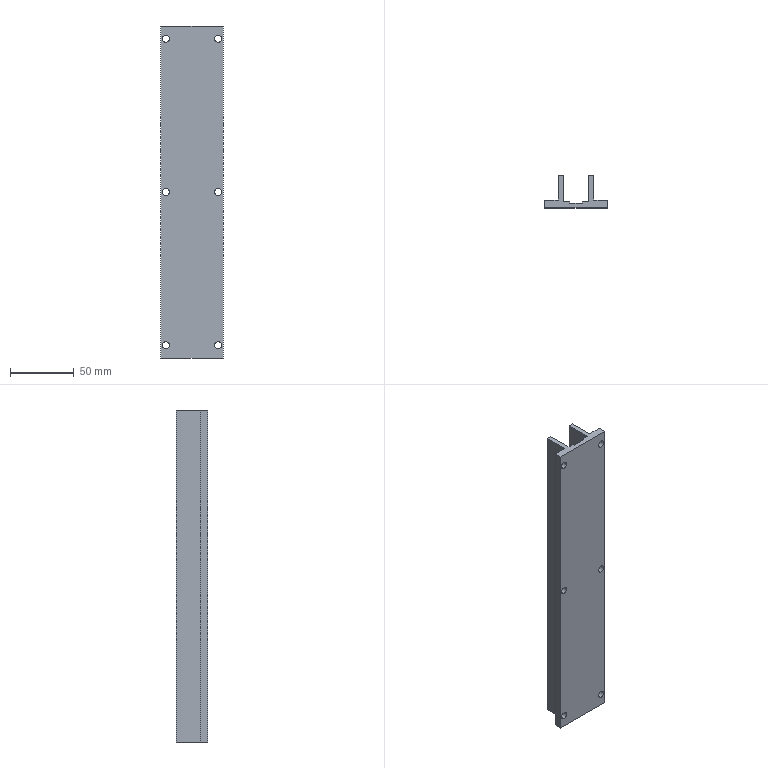Part | SolidWorks | features BaseBody 1 | 1 solid | 30 faces | box 49 x 25 x 260 mm | volume 106005 mm3 | plane 18 | cylinder 12 | commonest cylinder face diameters 5.5 x12
STEP:
#1=CARTESIAN_POINT('',(20.5,0.,252.75));
#2=VERTEX_POINT('',#1);
#3=CARTESIAN_POINT('',(20.5,0.,247.25));
#4=VERTEX_POINT('',#3);
#5=CARTESIAN_POINT('',(20.5,0.,250.));
#6=DIRECTION('',(0.,-1.,0.));
#7=DIRECTION('',(0.,0.,1.));
#8=AXIS2_PLACEMENT_3D('',#5,#6,#7);
#9=CIRCLE('',#8,2.75);
#10=EDGE_CURVE('',#2,#4,#9,.T.);
#11=ORIENTED_EDGE('',*,*,#10,.T.);
#12=CARTESIAN_POINT('',(20.5,6.,247.25));
#13=VERTEX_POINT('',#12);
#14=CARTESIAN_POINT('',(20.5,6.,247.25));
#15=DIRECTION('',(0.,1.,0.));
#16=VECTOR('',#15,1000.);
#17=LINE('',#14,#16);
#18=EDGE_CURVE('',#4,#13,#17,.T.);
#19=ORIENTED_EDGE('',*,*,#18,.T.);
#20=CARTESIAN_POINT('',(20.5,6.,252.75));
#21=VERTEX_POINT('',#20);
#22=CARTESIAN_POINT('',(20.5,6.,250.));
#23=DIRECTION('',(0.,-1.,0.));
#24=DIRECTION('',(0.,0.,1.));
#25=AXIS2_PLACEMENT_3D('',#22,#23,#24);
#26=CIRCLE('',#25,2.75);
#27=EDGE_CURVE('',#21,#13,#26,.T.);
#28=ORIENTED_EDGE('',*,*,#27,.F.);
#29=CARTESIAN_POINT('',(20.5,6.,252.75));
#30=DIRECTION('',(0.,1.,0.));
#31=VECTOR('',#30,1000.);
#32=LINE('',#29,#31);
#33=EDGE_CURVE('',#2,#21,#32,.T.);
#34=ORIENTED_EDGE('',*,*,#33,.F.);
#35=EDGE_LOOP('',(#11,#19,#28,#34));
#36=FACE_OUTER_BOUND('',#35,.T.);
#37=CARTESIAN_POINT('',(20.5,6.,250.));
#38=DIRECTION('',(0.,1.,0.));
#39=DIRECTION('',(0.,0.,1.));
#40=AXIS2_PLACEMENT_3D('',#37,#38,#39);
#41=CYLINDRICAL_SURFACE('',#40,2.75);
#42=ADVANCED_FACE('',(#36),#41,.F.);
#43=CARTESIAN_POINT('',(20.5,0.,132.75));
#44=VERTEX_POINT('',#43);
#45=CARTESIAN_POINT('',(20.5,0.,127.25));
#46=VERTEX_POINT('',#45);
#47=CARTESIAN_POINT('',(20.5,0.,130.));
#48=DIRECTION('',(0.,-1.,0.));
#49=DIRECTION('',(0.,0.,1.));
#50=AXIS2_PLACEMENT_3D('',#47,#48,#49);
#51=CIRCLE('',#50,2.75);
#52=EDGE_CURVE('',#44,#46,#51,.T.);
#53=ORIENTED_EDGE('',*,*,#52,.T.);
#54=CARTESIAN_POINT('',(20.5,6.,127.25));
#55=VERTEX_POINT('',#54);
#56=CARTESIAN_POINT('',(20.5,6.,127.25));
#57=DIRECTION('',(0.,1.,0.));
#58=VECTOR('',#57,1000.);
#59=LINE('',#56,#58);
#60=EDGE_CURVE('',#46,#55,#59,.T.);
#61=ORIENTED_EDGE('',*,*,#60,.T.);
#62=CARTESIAN_POINT('',(20.5,6.,132.75));
#63=VERTEX_POINT('',#62);
#64=CARTESIAN_POINT('',(20.5,6.,130.));
#65=DIRECTION('',(0.,-1.,0.));
#66=DIRECTION('',(0.,0.,1.));
#67=AXIS2_PLACEMENT_3D('',#64,#65,#66);
#68=CIRCLE('',#67,2.75);
#69=EDGE_CURVE('',#63,#55,#68,.T.);
#70=ORIENTED_EDGE('',*,*,#69,.F.);
#71=CARTESIAN_POINT('',(20.5,6.,132.75));
#72=DIRECTION('',(0.,1.,0.));
#73=VECTOR('',#72,1000.);
#74=LINE('',#71,#73);
#75=EDGE_CURVE('',#44,#63,#74,.T.);
#76=ORIENTED_EDGE('',*,*,#75,.F.);
#77=EDGE_LOOP('',(#53,#61,#70,#76));
#78=FACE_OUTER_BOUND('',#77,.T.);
#79=CARTESIAN_POINT('',(20.5,6.,130.));
#80=DIRECTION('',(0.,1.,0.));
#81=DIRECTION('',(0.,0.,1.));
#82=AXIS2_PLACEMENT_3D('',#79,#80,#81);
#83=CYLINDRICAL_SURFACE('',#82,2.75);
#84=ADVANCED_FACE('',(#78),#83,.F.);
#85=CARTESIAN_POINT('',(20.5,0.,12.75));
#86=VERTEX_POINT('',#85);
#87=CARTESIAN_POINT('',(20.5,0.,7.25));
#88=VERTEX_POINT('',#87);
#89=CARTESIAN_POINT('',(20.5,0.,10.));
#90=DIRECTION('',(0.,-1.,0.));
#91=DIRECTION('',(0.,0.,1.));
#92=AXIS2_PLACEMENT_3D('',#89,#90,#91);
#93=CIRCLE('',#92,2.75);
#94=EDGE_CURVE('',#86,#88,#93,.T.);
#95=ORIENTED_EDGE('',*,*,#94,.T.);
#96=CARTESIAN_POINT('',(20.5,6.,7.25));
#97=VERTEX_POINT('',#96);
#98=CARTESIAN_POINT('',(20.5,6.,7.25));
#99=DIRECTION('',(0.,1.,0.));
#100=VECTOR('',#99,1000.);
#101=LINE('',#98,#100);
#102=EDGE_CURVE('',#88,#97,#101,.T.);
#103=ORIENTED_EDGE('',*,*,#102,.T.);
#104=CARTESIAN_POINT('',(20.5,6.,12.75));
#105=VERTEX_POINT('',#104);
#106=CARTESIAN_POINT('',(20.5,6.,10.));
#107=DIRECTION('',(0.,-1.,0.));
#108=DIRECTION('',(0.,0.,1.));
#109=AXIS2_PLACEMENT_3D('',#106,#107,#108);
#110=CIRCLE('',#109,2.75);
#111=EDGE_CURVE('',#105,#97,#110,.T.);
#112=ORIENTED_EDGE('',*,*,#111,.F.);
#113=CARTESIAN_POINT('',(20.5,6.,12.75));
#114=DIRECTION('',(0.,1.,0.));
#115=VECTOR('',#114,1000.);
#116=LINE('',#113,#115);
#117=EDGE_CURVE('',#86,#105,#116,.T.);
#118=ORIENTED_EDGE('',*,*,#117,.F.);
#119=EDGE_LOOP('',(#95,#103,#112,#118));
#120=FACE_OUTER_BOUND('',#119,.T.);
#121=CARTESIAN_POINT('',(20.5,6.,10.));
#122=DIRECTION('',(0.,1.,0.));
#123=DIRECTION('',(0.,0.,1.));
#124=AXIS2_PLACEMENT_3D('',#121,#122,#123);
#125=CYLINDRICAL_SURFACE('',#124,2.75);
#126=ADVANCED_FACE('',(#120),#125,.F.);
#127=CARTESIAN_POINT('',(-20.5,0.,12.75));
#128=VERTEX_POINT('',#127);
#129=CARTESIAN_POINT('',(-20.5,0.,7.25));
#130=VERTEX_POINT('',#129);
#131=CARTESIAN_POINT('',(-20.5,0.,10.));
#132=DIRECTION('',(0.,-1.,0.));
#133=DIRECTION('',(0.,0.,1.));
#134=AXIS2_PLACEMENT_3D('',#131,#132,#133);
#135=CIRCLE('',#134,2.75);
#136=EDGE_CURVE('',#128,#130,#135,.T.);
#137=ORIENTED_EDGE('',*,*,#136,.T.);
#138=CARTESIAN_POINT('',(-20.5,6.,7.25));
#139=VERTEX_POINT('',#138);
#140=CARTESIAN_POINT('',(-20.5,6.,7.25));
#141=DIRECTION('',(0.,1.,0.));
#142=VECTOR('',#141,1000.);
#143=LINE('',#140,#142);
#144=EDGE_CURVE('',#130,#139,#143,.T.);
#145=ORIENTED_EDGE('',*,*,#144,.T.);
#146=CARTESIAN_POINT('',(-20.5,6.,12.75));
#147=VERTEX_POINT('',#146);
#148=CARTESIAN_POINT('',(-20.5,6.,10.));
#149=DIRECTION('',(0.,-1.,0.));
#150=DIRECTION('',(0.,0.,1.));
#151=AXIS2_PLACEMENT_3D('',#148,#149,#150);
#152=CIRCLE('',#151,2.75);
#153=EDGE_CURVE('',#147,#139,#152,.T.);
#154=ORIENTED_EDGE('',*,*,#153,.F.);
#155=CARTESIAN_POINT('',(-20.5,6.,12.75));
#156=DIRECTION('',(0.,1.,0.));
#157=VECTOR('',#156,1000.);
#158=LINE('',#155,#157);
#159=EDGE_CURVE('',#128,#147,#158,.T.);
#160=ORIENTED_EDGE('',*,*,#159,.F.);
#161=EDGE_LOOP('',(#137,#145,#154,#160));
#162=FACE_OUTER_BOUND('',#161,.T.);
#163=CARTESIAN_POINT('',(-20.5,6.,10.));
#164=DIRECTION('',(0.,1.,0.));
#165=DIRECTION('',(0.,0.,1.));
#166=AXIS2_PLACEMENT_3D('',#163,#164,#165);
#167=CYLINDRICAL_SURFACE('',#166,2.75);
#168=ADVANCED_FACE('',(#162),#167,.F.);
#169=CARTESIAN_POINT('',(-20.5,0.,132.75));
#170=VERTEX_POINT('',#169);
#171=CARTESIAN_POINT('',(-20.5,0.,127.25));
#172=VERTEX_POINT('',#171);
#173=CARTESIAN_POINT('',(-20.5,0.,130.));
#174=DIRECTION('',(0.,-1.,0.));
#175=DIRECTION('',(0.,0.,1.));
#176=AXIS2_PLACEMENT_3D('',#173,#174,#175);
#177=CIRCLE('',#176,2.75);
#178=EDGE_CURVE('',#170,#172,#177,.T.);
#179=ORIENTED_EDGE('',*,*,#178,.T.);
#180=CARTESIAN_POINT('',(-20.5,6.,127.25));
#181=VERTEX_POINT('',#180);
#182=CARTESIAN_POINT('',(-20.5,6.,127.25));
#183=DIRECTION('',(0.,1.,0.));
#184=VECTOR('',#183,1000.);
#185=LINE('',#182,#184);
#186=EDGE_CURVE('',#172,#181,#185,.T.);
#187=ORIENTED_EDGE('',*,*,#186,.T.);
#188=CARTESIAN_POINT('',(-20.5,6.,132.75));
#189=VERTEX_POINT('',#188);
#190=CARTESIAN_POINT('',(-20.5,6.,130.));
#191=DIRECTION('',(0.,-1.,0.));
#192=DIRECTION('',(0.,0.,1.));
#193=AXIS2_PLACEMENT_3D('',#190,#191,#192);
#194=CIRCLE('',#193,2.75);
#195=EDGE_CURVE('',#189,#181,#194,.T.);
#196=ORIENTED_EDGE('',*,*,#195,.F.);
#197=CARTESIAN_POINT('',(-20.5,6.,132.75));
#198=DIRECTION('',(0.,1.,0.));
#199=VECTOR('',#198,1000.);
#200=LINE('',#197,#199);
#201=EDGE_CURVE('',#170,#189,#200,.T.);
#202=ORIENTED_EDGE('',*,*,#201,.F.);
#203=EDGE_LOOP('',(#179,#187,#196,#202));
#204=FACE_OUTER_BOUND('',#203,.T.);
#205=CARTESIAN_POINT('',(-20.5,6.,130.));
#206=DIRECTION('',(0.,1.,0.));
#207=DIRECTION('',(0.,0.,1.));
#208=AXIS2_PLACEMENT_3D('',#205,#206,#207);
#209=CYLINDRICAL_SURFACE('',#208,2.75);
#210=ADVANCED_FACE('',(#204),#209,.F.);
#211=CARTESIAN_POINT('',(-20.5,0.,252.75));
#212=VERTEX_POINT('',#211);
#213=CARTESIAN_POINT('',(-20.5,0.,247.25));
#214=VERTEX_POINT('',#213);
#215=CARTESIAN_POINT('',(-20.5,0.,250.));
#216=DIRECTION('',(0.,-1.,0.));
#217=DIRECTION('',(0.,0.,1.));
#218=AXIS2_PLACEMENT_3D('',#215,#216,#217);
#219=CIRCLE('',#218,2.75);
#220=EDGE_CURVE('',#212,#214,#219,.T.);
#221=ORIENTED_EDGE('',*,*,#220,.T.);
#222=CARTESIAN_POINT('',(-20.5,6.,247.25));
#223=VERTEX_POINT('',#222);
#224=CARTESIAN_POINT('',(-20.5,6.,247.25));
#225=DIRECTION('',(0.,1.,0.));
#226=VECTOR('',#225,1000.);
#227=LINE('',#224,#226);
#228=EDGE_CURVE('',#214,#223,#227,.T.);
#229=ORIENTED_EDGE('',*,*,#228,.T.);
#230=CARTESIAN_POINT('',(-20.5,6.,252.75));
#231=VERTEX_POINT('',#230);
#232=CARTESIAN_POINT('',(-20.5,6.,250.));
#233=DIRECTION('',(0.,-1.,0.));
#234=DIRECTION('',(0.,0.,1.));
#235=AXIS2_PLACEMENT_3D('',#232,#233,#234);
#236=CIRCLE('',#235,2.75);
#237=EDGE_CURVE('',#231,#223,#236,.T.);
#238=ORIENTED_EDGE('',*,*,#237,.F.);
#239=CARTESIAN_POINT('',(-20.5,6.,252.75));
#240=DIRECTION('',(0.,1.,0.));
#241=VECTOR('',#240,1000.);
#242=LINE('',#239,#241);
#243=EDGE_CURVE('',#212,#231,#242,.T.);
#244=ORIENTED_EDGE('',*,*,#243,.F.);
#245=EDGE_LOOP('',(#221,#229,#238,#244));
#246=FACE_OUTER_BOUND('',#245,.T.);
#247=CARTESIAN_POINT('',(-20.5,6.,250.));
#248=DIRECTION('',(0.,1.,0.));
#249=DIRECTION('',(0.,0.,1.));
#250=AXIS2_PLACEMENT_3D('',#247,#248,#249);
#251=CYLINDRICAL_SURFACE('',#250,2.75);
#252=ADVANCED_FACE('',(#246),#251,.F.);
#253=CARTESIAN_POINT('',(24.5,0.,260.));
#254=VERTEX_POINT('',#253);
#255=CARTESIAN_POINT('',(24.5,0.,0.));
#256=VERTEX_POINT('',#255);
#257=CARTESIAN_POINT('',(24.5,0.,260.));
#258=DIRECTION('',(0.,0.,-1.));
#259=VECTOR('',#258,1000.);
#260=LINE('',#257,#259);
#261=EDGE_CURVE('',#254,#256,#260,.T.);
#262=ORIENTED_EDGE('',*,*,#261,.F.);
#263=CARTESIAN_POINT('',(-24.5,0.,260.));
#264=VERTEX_POINT('',#263);
#265=CARTESIAN_POINT('',(-24.5,0.,260.));
#266=DIRECTION('',(1.,0.,0.));
#267=VECTOR('',#266,1000.);
#268=LINE('',#265,#267);
#269=EDGE_CURVE('',#264,#254,#268,.T.);
#270=ORIENTED_EDGE('',*,*,#269,.F.);
#271=CARTESIAN_POINT('',(-24.5,0.,0.));
#272=VERTEX_POINT('',#271);
#273=CARTESIAN_POINT('',(-24.5,0.,260.));
#274=DIRECTION('',(0.,0.,1.));
#275=VECTOR('',#274,1000.);
#276=LINE('',#273,#275);
#277=EDGE_CURVE('',#272,#264,#276,.T.);
#278=ORIENTED_EDGE('',*,*,#277,.F.);
#279=CARTESIAN_POINT('',(-24.5,0.,0.));
#280=DIRECTION('',(-1.,0.,0.));
#281=VECTOR('',#280,1000.);
#282=LINE('',#279,#281);
#283=EDGE_CURVE('',#256,#272,#282,.T.);
#284=ORIENTED_EDGE('',*,*,#283,.F.);
#285=EDGE_LOOP('',(#262,#270,#278,#284));
#286=FACE_OUTER_BOUND('',#285,.T.);
#287=ORIENTED_EDGE('',*,*,#10,.F.);
#288=CARTESIAN_POINT('',(20.5,0.,250.));
#289=DIRECTION('',(0.,-1.,0.));
#290=DIRECTION('',(0.,0.,1.));
#291=AXIS2_PLACEMENT_3D('',#288,#289,#290);
#292=CIRCLE('',#291,2.75);
#293=EDGE_CURVE('',#4,#2,#292,.T.);
#294=ORIENTED_EDGE('',*,*,#293,.F.);
#295=EDGE_LOOP('',(#287,#294));
#296=FACE_BOUND('',#295,.T.);
#297=ORIENTED_EDGE('',*,*,#52,.F.);
#298=CARTESIAN_POINT('',(20.5,0.,130.));
#299=DIRECTION('',(0.,-1.,0.));
#300=DIRECTION('',(0.,0.,1.));
#301=AXIS2_PLACEMENT_3D('',#298,#299,#300);
#302=CIRCLE('',#301,2.75);
#303=EDGE_CURVE('',#46,#44,#302,.T.);
#304=ORIENTED_EDGE('',*,*,#303,.F.);
#305=EDGE_LOOP('',(#297,#304));
#306=FACE_BOUND('',#305,.T.);
#307=ORIENTED_EDGE('',*,*,#94,.F.);
#308=CARTESIAN_POINT('',(20.5,0.,10.));
#309=DIRECTION('',(0.,-1.,0.));
#310=DIRECTION('',(0.,0.,1.));
#311=AXIS2_PLACEMENT_3D('',#308,#309,#310);
#312=CIRCLE('',#311,2.75);
#313=EDGE_CURVE('',#88,#86,#312,.T.);
#314=ORIENTED_EDGE('',*,*,#313,.F.);
#315=EDGE_LOOP('',(#307,#314));
#316=FACE_BOUND('',#315,.T.);
#317=ORIENTED_EDGE('',*,*,#136,.F.);
#318=CARTESIAN_POINT('',(-20.5,0.,10.));
#319=DIRECTION('',(0.,-1.,0.));
#320=DIRECTION('',(0.,0.,1.));
#321=AXIS2_PLACEMENT_3D('',#318,#319,#320);
#322=CIRCLE('',#321,2.75);
#323=EDGE_CURVE('',#130,#128,#322,.T.);
#324=ORIENTED_EDGE('',*,*,#323,.F.);
#325=EDGE_LOOP('',(#317,#324));
#326=FACE_BOUND('',#325,.T.);
#327=ORIENTED_EDGE('',*,*,#178,.F.);
#328=CARTESIAN_POINT('',(-20.5,0.,130.));
#329=DIRECTION('',(0.,-1.,0.));
#330=DIRECTION('',(0.,0.,1.));
#331=AXIS2_PLACEMENT_3D('',#328,#329,#330);
#332=CIRCLE('',#331,2.75);
#333=EDGE_CURVE('',#172,#170,#332,.T.);
#334=ORIENTED_EDGE('',*,*,#333,.F.);
#335=EDGE_LOOP('',(#327,#334));
#336=FACE_BOUND('',#335,.T.);
#337=ORIENTED_EDGE('',*,*,#220,.F.);
#338=CARTESIAN_POINT('',(-20.5,0.,250.));
#339=DIRECTION('',(0.,-1.,0.));
#340=DIRECTION('',(0.,0.,1.));
#341=AXIS2_PLACEMENT_3D('',#338,#339,#340);
#342=CIRCLE('',#341,2.75);
#343=EDGE_CURVE('',#214,#212,#342,.T.);
#344=ORIENTED_EDGE('',*,*,#343,.F.);
#345=EDGE_LOOP('',(#337,#344));
#346=FACE_BOUND('',#345,.T.);
#347=CARTESIAN_POINT('',(-24.5,0.,260.));
#348=DIRECTION('',(0.,1.,0.));
#349=DIRECTION('',(0.,0.,1.));
#350=AXIS2_PLACEMENT_3D('',#347,#348,#349);
#351=PLANE('',#350);
#352=ADVANCED_FACE('',(#286,#296,#306,#316,#326,#336,#346),#351,.F.);
#353=ORIENTED_EDGE('',*,*,#283,.T.);
#354=CARTESIAN_POINT('',(-24.5,6.,0.));
#355=VERTEX_POINT('',#354);
#356=CARTESIAN_POINT('',(-24.5,0.,0.));
#357=DIRECTION('',(0.,-1.,0.));
#358=VECTOR('',#357,1000.);
#359=LINE('',#356,#358);
#360=EDGE_CURVE('',#355,#272,#359,.T.);
#361=ORIENTED_EDGE('',*,*,#360,.F.);
#362=CARTESIAN_POINT('',(-14.,6.,0.));
#363=VERTEX_POINT('',#362);
#364=CARTESIAN_POINT('',(0.,6.,0.));
#365=DIRECTION('',(-1.,0.,0.));
#366=VECTOR('',#365,1000.);
#367=LINE('',#364,#366);
#368=EDGE_CURVE('',#363,#355,#367,.T.);
#369=ORIENTED_EDGE('',*,*,#368,.F.);
#370=CARTESIAN_POINT('',(-14.,25.,0.));
#371=VERTEX_POINT('',#370);
#372=CARTESIAN_POINT('',(-14.,0.,0.));
#373=DIRECTION('',(0.,-1.,0.));
#374=VECTOR('',#373,1000.);
#375=LINE('',#372,#374);
#376=EDGE_CURVE('',#371,#363,#375,.T.);
#377=ORIENTED_EDGE('',*,*,#376,.F.);
#378=CARTESIAN_POINT('',(-10.,25.,0.));
#379=VERTEX_POINT('',#378);
#380=CARTESIAN_POINT('',(0.,25.,0.));
#381=DIRECTION('',(-1.,0.,0.));
#382=VECTOR('',#381,1000.);
#383=LINE('',#380,#382);
#384=EDGE_CURVE('',#379,#371,#383,.T.);
#385=ORIENTED_EDGE('',*,*,#384,.F.);
#386=CARTESIAN_POINT('',(-10.,5.,0.));
#387=VERTEX_POINT('',#386);
#388=CARTESIAN_POINT('',(-10.,0.,0.));
#389=DIRECTION('',(0.,1.,0.));
#390=VECTOR('',#389,1000.);
#391=LINE('',#388,#390);
#392=EDGE_CURVE('',#387,#379,#391,.T.);
#393=ORIENTED_EDGE('',*,*,#392,.F.);
#394=CARTESIAN_POINT('',(-5.,5.,0.));
#395=VERTEX_POINT('',#394);
#396=CARTESIAN_POINT('',(0.,5.,0.));
#397=DIRECTION('',(-1.,0.,0.));
#398=VECTOR('',#397,1000.);
#399=LINE('',#396,#398);
#400=EDGE_CURVE('',#395,#387,#399,.T.);
#401=ORIENTED_EDGE('',*,*,#400,.F.);
#402=CARTESIAN_POINT('',(-5.,3.5,0.));
#403=VERTEX_POINT('',#402);
#404=CARTESIAN_POINT('',(-5.,5.,0.));
#405=DIRECTION('',(0.,-1.,0.));
#406=VECTOR('',#405,1000.);
#407=LINE('',#404,#406);
#408=EDGE_CURVE('',#395,#403,#407,.T.);
#409=ORIENTED_EDGE('',*,*,#408,.T.);
#410=CARTESIAN_POINT('',(5.,3.5,0.));
#411=VERTEX_POINT('',#410);
#412=CARTESIAN_POINT('',(0.,3.5,0.));
#413=DIRECTION('',(-1.,0.,0.));
#414=VECTOR('',#413,1000.);
#415=LINE('',#412,#414);
#416=EDGE_CURVE('',#411,#403,#415,.T.);
#417=ORIENTED_EDGE('',*,*,#416,.F.);
#418=CARTESIAN_POINT('',(5.,5.,0.));
#419=VERTEX_POINT('',#418);
#420=CARTESIAN_POINT('',(5.,5.,0.));
#421=DIRECTION('',(0.,1.,0.));
#422=VECTOR('',#421,1000.);
#423=LINE('',#420,#422);
#424=EDGE_CURVE('',#411,#419,#423,.T.);
#425=ORIENTED_EDGE('',*,*,#424,.T.);
#426=CARTESIAN_POINT('',(10.,5.,0.));
#427=VERTEX_POINT('',#426);
#428=CARTESIAN_POINT('',(0.,5.,0.));
#429=DIRECTION('',(-1.,0.,0.));
#430=VECTOR('',#429,1000.);
#431=LINE('',#428,#430);
#432=EDGE_CURVE('',#427,#419,#431,.T.);
#433=ORIENTED_EDGE('',*,*,#432,.F.);
#434=CARTESIAN_POINT('',(10.,25.,0.));
#435=VERTEX_POINT('',#434);
#436=CARTESIAN_POINT('',(10.,0.,0.));
#437=DIRECTION('',(0.,-1.,0.));
#438=VECTOR('',#437,1000.);
#439=LINE('',#436,#438);
#440=EDGE_CURVE('',#435,#427,#439,.T.);
#441=ORIENTED_EDGE('',*,*,#440,.F.);
#442=CARTESIAN_POINT('',(14.,25.,0.));
#443=VERTEX_POINT('',#442);
#444=CARTESIAN_POINT('',(0.,25.,0.));
#445=DIRECTION('',(-1.,0.,0.));
#446=VECTOR('',#445,1000.);
#447=LINE('',#444,#446);
#448=EDGE_CURVE('',#443,#435,#447,.T.);
#449=ORIENTED_EDGE('',*,*,#448,.F.);
#450=CARTESIAN_POINT('',(14.,6.,0.));
#451=VERTEX_POINT('',#450);
#452=CARTESIAN_POINT('',(14.,0.,0.));
#453=DIRECTION('',(0.,1.,0.));
#454=VECTOR('',#453,1000.);
#455=LINE('',#452,#454);
#456=EDGE_CURVE('',#451,#443,#455,.T.);
#457=ORIENTED_EDGE('',*,*,#456,.F.);
#458=CARTESIAN_POINT('',(24.5,6.,0.));
#459=VERTEX_POINT('',#458);
#460=CARTESIAN_POINT('',(0.,6.,0.));
#461=DIRECTION('',(-1.,0.,0.));
#462=VECTOR('',#461,1000.);
#463=LINE('',#460,#462);
#464=EDGE_CURVE('',#459,#451,#463,.T.);
#465=ORIENTED_EDGE('',*,*,#464,.F.);
#466=CARTESIAN_POINT('',(24.5,0.,0.));
#467=DIRECTION('',(0.,1.,0.));
#468=VECTOR('',#467,1000.);
#469=LINE('',#466,#468);
#470=EDGE_CURVE('',#256,#459,#469,.T.);
#471=ORIENTED_EDGE('',*,*,#470,.F.);
#472=EDGE_LOOP('',(#353,#361,#369,#377,#385,#393,#401,#409,#417,#425,#433,#441,#449,#457,#465,#471));
#473=FACE_OUTER_BOUND('',#472,.T.);
#474=CARTESIAN_POINT('',(0.,0.,0.));
#475=DIRECTION('',(0.,0.,1.));
#476=DIRECTION('',(1.,0.,0.));
#477=AXIS2_PLACEMENT_3D('',#474,#475,#476);
#478=PLANE('',#477);
#479=ADVANCED_FACE('',(#473),#478,.F.);
#480=CARTESIAN_POINT('',(24.5,6.,260.));
#481=VERTEX_POINT('',#480);
#482=CARTESIAN_POINT('',(24.5,6.,260.));
#483=DIRECTION('',(0.,0.,-1.));
#484=VECTOR('',#483,1000.);
#485=LINE('',#482,#484);
#486=EDGE_CURVE('',#481,#459,#485,.T.);
#487=ORIENTED_EDGE('',*,*,#486,.F.);
#488=CARTESIAN_POINT('',(24.5,0.,260.));
#489=DIRECTION('',(0.,1.,0.));
#490=VECTOR('',#489,1000.);
#491=LINE('',#488,#490);
#492=EDGE_CURVE('',#254,#481,#491,.T.);
#493=ORIENTED_EDGE('',*,*,#492,.F.);
#494=ORIENTED_EDGE('',*,*,#261,.T.);
#495=ORIENTED_EDGE('',*,*,#470,.T.);
#496=EDGE_LOOP('',(#487,#493,#494,#495));
#497=FACE_OUTER_BOUND('',#496,.T.);
#498=CARTESIAN_POINT('',(24.5,0.,260.));
#499=DIRECTION('',(-1.,0.,0.));
#500=DIRECTION('',(0.,0.,1.));
#501=AXIS2_PLACEMENT_3D('',#498,#499,#500);
#502=PLANE('',#501);
#503=ADVANCED_FACE('',(#497),#502,.F.);
#504=CARTESIAN_POINT('',(-24.5,6.,260.));
#505=VERTEX_POINT('',#504);
#506=CARTESIAN_POINT('',(-24.5,0.,260.));
#507=DIRECTION('',(0.,-1.,0.));
#508=VECTOR('',#507,1000.);
#509=LINE('',#506,#508);
#510=EDGE_CURVE('',#505,#264,#509,.T.);
#511=ORIENTED_EDGE('',*,*,#510,.T.);
#512=ORIENTED_EDGE('',*,*,#269,.T.);
#513=ORIENTED_EDGE('',*,*,#492,.T.);
#514=CARTESIAN_POINT('',(14.,6.,260.));
#515=VERTEX_POINT('',#514);
#516=CARTESIAN_POINT('',(0.,6.,260.));
#517=DIRECTION('',(-1.,0.,0.));
#518=VECTOR('',#517,1000.);
#519=LINE('',#516,#518);
#520=EDGE_CURVE('',#481,#515,#519,.T.);
#521=ORIENTED_EDGE('',*,*,#520,.T.);
#522=CARTESIAN_POINT('',(14.,25.,260.));
#523=VERTEX_POINT('',#522);
#524=CARTESIAN_POINT('',(14.,0.,260.));
#525=DIRECTION('',(0.,1.,0.));
#526=VECTOR('',#525,1000.);
#527=LINE('',#524,#526);
#528=EDGE_CURVE('',#515,#523,#527,.T.);
#529=ORIENTED_EDGE('',*,*,#528,.T.);
#530=CARTESIAN_POINT('',(10.,25.,260.));
#531=VERTEX_POINT('',#530);
#532=CARTESIAN_POINT('',(0.,25.,260.));
#533=DIRECTION('',(-1.,0.,0.));
#534=VECTOR('',#533,1000.);
#535=LINE('',#532,#534);
#536=EDGE_CURVE('',#523,#531,#535,.T.);
#537=ORIENTED_EDGE('',*,*,#536,.T.);
#538=CARTESIAN_POINT('',(10.,5.,260.));
#539=VERTEX_POINT('',#538);
#540=CARTESIAN_POINT('',(10.,0.,260.));
#541=DIRECTION('',(0.,-1.,0.));
#542=VECTOR('',#541,1000.);
#543=LINE('',#540,#542);
#544=EDGE_CURVE('',#531,#539,#543,.T.);
#545=ORIENTED_EDGE('',*,*,#544,.T.);
#546=CARTESIAN_POINT('',(5.,5.,260.));
#547=VERTEX_POINT('',#546);
#548=CARTESIAN_POINT('',(0.,5.,260.));
#549=DIRECTION('',(-1.,0.,0.));
#550=VECTOR('',#549,1000.);
#551=LINE('',#548,#550);
#552=EDGE_CURVE('',#539,#547,#551,.T.);
#553=ORIENTED_EDGE('',*,*,#552,.T.);
#554=CARTESIAN_POINT('',(5.,3.5,260.));
#555=VERTEX_POINT('',#554);
#556=CARTESIAN_POINT('',(5.,5.,260.));
#557=DIRECTION('',(0.,-1.,0.));
#558=VECTOR('',#557,1000.);
#559=LINE('',#556,#558);
#560=EDGE_CURVE('',#547,#555,#559,.T.);
#561=ORIENTED_EDGE('',*,*,#560,.T.);
#562=CARTESIAN_POINT('',(-5.,3.5,260.));
#563=VERTEX_POINT('',#562);
#564=CARTESIAN_POINT('',(0.,3.5,260.));
#565=DIRECTION('',(-1.,0.,0.));
#566=VECTOR('',#565,1000.);
#567=LINE('',#564,#566);
#568=EDGE_CURVE('',#555,#563,#567,.T.);
#569=ORIENTED_EDGE('',*,*,#568,.T.);
#570=CARTESIAN_POINT('',(-5.,5.,260.));
#571=VERTEX_POINT('',#570);
#572=CARTESIAN_POINT('',(-5.,5.,260.));
#573=DIRECTION('',(0.,1.,0.));
#574=VECTOR('',#573,1000.);
#575=LINE('',#572,#574);
#576=EDGE_CURVE('',#563,#571,#575,.T.);
#577=ORIENTED_EDGE('',*,*,#576,.T.);
#578=CARTESIAN_POINT('',(-10.,5.,260.));
#579=VERTEX_POINT('',#578);
#580=CARTESIAN_POINT('',(0.,5.,260.));
#581=DIRECTION('',(-1.,0.,0.));
#582=VECTOR('',#581,1000.);
#583=LINE('',#580,#582);
#584=EDGE_CURVE('',#571,#579,#583,.T.);
#585=ORIENTED_EDGE('',*,*,#584,.T.);
#586=CARTESIAN_POINT('',(-10.,25.,260.));
#587=VERTEX_POINT('',#586);
#588=CARTESIAN_POINT('',(-10.,0.,260.));
#589=DIRECTION('',(0.,1.,0.));
#590=VECTOR('',#589,1000.);
#591=LINE('',#588,#590);
#592=EDGE_CURVE('',#579,#587,#591,.T.);
#593=ORIENTED_EDGE('',*,*,#592,.T.);
#594=CARTESIAN_POINT('',(-14.,25.,260.));
#595=VERTEX_POINT('',#594);
#596=CARTESIAN_POINT('',(0.,25.,260.));
#597=DIRECTION('',(-1.,0.,0.));
#598=VECTOR('',#597,1000.);
#599=LINE('',#596,#598);
#600=EDGE_CURVE('',#587,#595,#599,.T.);
#601=ORIENTED_EDGE('',*,*,#600,.T.);
#602=CARTESIAN_POINT('',(-14.,6.,260.));
#603=VERTEX_POINT('',#602);
#604=CARTESIAN_POINT('',(-14.,0.,260.));
#605=DIRECTION('',(0.,-1.,0.));
#606=VECTOR('',#605,1000.);
#607=LINE('',#604,#606);
#608=EDGE_CURVE('',#595,#603,#607,.T.);
#609=ORIENTED_EDGE('',*,*,#608,.T.);
#610=CARTESIAN_POINT('',(0.,6.,260.));
#611=DIRECTION('',(-1.,0.,0.));
#612=VECTOR('',#611,1000.);
#613=LINE('',#610,#612);
#614=EDGE_CURVE('',#603,#505,#613,.T.);
#615=ORIENTED_EDGE('',*,*,#614,.T.);
#616=EDGE_LOOP('',(#511,#512,#513,#521,#529,#537,#545,#553,#561,#569,#577,#585,#593,#601,#609,#615));
#617=FACE_OUTER_BOUND('',#616,.T.);
#618=CARTESIAN_POINT('',(0.,0.,260.));
#619=DIRECTION('',(0.,0.,1.));
#620=DIRECTION('',(1.,0.,0.));
#621=AXIS2_PLACEMENT_3D('',#618,#619,#620);
#622=PLANE('',#621);
#623=ADVANCED_FACE('',(#617),#622,.T.);
#624=ORIENTED_EDGE('',*,*,#277,.T.);
#625=ORIENTED_EDGE('',*,*,#510,.F.);
#626=CARTESIAN_POINT('',(-24.5,6.,260.));
#627=DIRECTION('',(0.,0.,1.));
#628=VECTOR('',#627,1000.);
#629=LINE('',#626,#628);
#630=EDGE_CURVE('',#355,#505,#629,.T.);
#631=ORIENTED_EDGE('',*,*,#630,.F.);
#632=ORIENTED_EDGE('',*,*,#360,.T.);
#633=EDGE_LOOP('',(#624,#625,#631,#632));
#634=FACE_OUTER_BOUND('',#633,.T.);
#635=CARTESIAN_POINT('',(-24.5,0.,260.));
#636=DIRECTION('',(1.,0.,0.));
#637=DIRECTION('',(0.,0.,-1.));
#638=AXIS2_PLACEMENT_3D('',#635,#636,#637);
#639=PLANE('',#638);
#640=ADVANCED_FACE('',(#634),#639,.F.);
#641=ORIENTED_EDGE('',*,*,#18,.F.);
#642=ORIENTED_EDGE('',*,*,#293,.T.);
#643=ORIENTED_EDGE('',*,*,#33,.T.);
#644=CARTESIAN_POINT('',(20.5,6.,250.));
#645=DIRECTION('',(0.,-1.,0.));
#646=DIRECTION('',(0.,0.,1.));
#647=AXIS2_PLACEMENT_3D('',#644,#645,#646);
#648=CIRCLE('',#647,2.75);
#649=EDGE_CURVE('',#13,#21,#648,.T.);
#650=ORIENTED_EDGE('',*,*,#649,.F.);
#651=EDGE_LOOP('',(#641,#642,#643,#650));
#652=FACE_OUTER_BOUND('',#651,.T.);
#653=CARTESIAN_POINT('',(20.5,6.,250.));
#654=DIRECTION('',(0.,1.,0.));
#655=DIRECTION('',(0.,0.,1.));
#656=AXIS2_PLACEMENT_3D('',#653,#654,#655);
#657=CYLINDRICAL_SURFACE('',#656,2.75);
#658=ADVANCED_FACE('',(#652),#657,.F.);
#659=ORIENTED_EDGE('',*,*,#60,.F.);
#660=ORIENTED_EDGE('',*,*,#303,.T.);
#661=ORIENTED_EDGE('',*,*,#75,.T.);
#662=CARTESIAN_POINT('',(20.5,6.,130.));
#663=DIRECTION('',(0.,-1.,0.));
#664=DIRECTION('',(0.,0.,1.));
#665=AXIS2_PLACEMENT_3D('',#662,#663,#664);
#666=CIRCLE('',#665,2.75);
#667=EDGE_CURVE('',#55,#63,#666,.T.);
#668=ORIENTED_EDGE('',*,*,#667,.F.);
#669=EDGE_LOOP('',(#659,#660,#661,#668));
#670=FACE_OUTER_BOUND('',#669,.T.);
#671=CARTESIAN_POINT('',(20.5,6.,130.));
#672=DIRECTION('',(0.,1.,0.));
#673=DIRECTION('',(0.,0.,1.));
#674=AXIS2_PLACEMENT_3D('',#671,#672,#673);
#675=CYLINDRICAL_SURFACE('',#674,2.75);
#676=ADVANCED_FACE('',(#670),#675,.F.);
#677=ORIENTED_EDGE('',*,*,#102,.F.);
#678=ORIENTED_EDGE('',*,*,#313,.T.);
#679=ORIENTED_EDGE('',*,*,#117,.T.);
#680=CARTESIAN_POINT('',(20.5,6.,10.));
#681=DIRECTION('',(0.,-1.,0.));
#682=DIRECTION('',(0.,0.,1.));
#683=AXIS2_PLACEMENT_3D('',#680,#681,#682);
#684=CIRCLE('',#683,2.75);
#685=EDGE_CURVE('',#97,#105,#684,.T.);
#686=ORIENTED_EDGE('',*,*,#685,.F.);
#687=EDGE_LOOP('',(#677,#678,#679,#686));
#688=FACE_OUTER_BOUND('',#687,.T.);
#689=CARTESIAN_POINT('',(20.5,6.,10.));
#690=DIRECTION('',(0.,1.,0.));
#691=DIRECTION('',(0.,0.,1.));
#692=AXIS2_PLACEMENT_3D('',#689,#690,#691);
#693=CYLINDRICAL_SURFACE('',#692,2.75);
#694=ADVANCED_FACE('',(#688),#693,.F.);
#695=ORIENTED_EDGE('',*,*,#144,.F.);
#696=ORIENTED_EDGE('',*,*,#323,.T.);
#697=ORIENTED_EDGE('',*,*,#159,.T.);
#698=CARTESIAN_POINT('',(-20.5,6.,10.));
#699=DIRECTION('',(0.,-1.,0.));
#700=DIRECTION('',(0.,0.,1.));
#701=AXIS2_PLACEMENT_3D('',#698,#699,#700);
#702=CIRCLE('',#701,2.75);
#703=EDGE_CURVE('',#139,#147,#702,.T.);
#704=ORIENTED_EDGE('',*,*,#703,.F.);
#705=EDGE_LOOP('',(#695,#696,#697,#704));
#706=FACE_OUTER_BOUND('',#705,.T.);
#707=CARTESIAN_POINT('',(-20.5,6.,10.));
#708=DIRECTION('',(0.,1.,0.));
#709=DIRECTION('',(0.,0.,1.));
#710=AXIS2_PLACEMENT_3D('',#707,#708,#709);
#711=CYLINDRICAL_SURFACE('',#710,2.75);
#712=ADVANCED_FACE('',(#706),#711,.F.);
#713=ORIENTED_EDGE('',*,*,#186,.F.);
#714=ORIENTED_EDGE('',*,*,#333,.T.);
#715=ORIENTED_EDGE('',*,*,#201,.T.);
#716=CARTESIAN_POINT('',(-20.5,6.,130.));
#717=DIRECTION('',(0.,-1.,0.));
#718=DIRECTION('',(0.,0.,1.));
#719=AXIS2_PLACEMENT_3D('',#716,#717,#718);
#720=CIRCLE('',#719,2.75);
#721=EDGE_CURVE('',#181,#189,#720,.T.);
#722=ORIENTED_EDGE('',*,*,#721,.F.);
#723=EDGE_LOOP('',(#713,#714,#715,#722));
#724=FACE_OUTER_BOUND('',#723,.T.);
#725=CARTESIAN_POINT('',(-20.5,6.,130.));
#726=DIRECTION('',(0.,1.,0.));
#727=DIRECTION('',(0.,0.,1.));
#728=AXIS2_PLACEMENT_3D('',#725,#726,#727);
#729=CYLINDRICAL_SURFACE('',#728,2.75);
#730=ADVANCED_FACE('',(#724),#729,.F.);
#731=ORIENTED_EDGE('',*,*,#228,.F.);
#732=ORIENTED_EDGE('',*,*,#343,.T.);
#733=ORIENTED_EDGE('',*,*,#243,.T.);
#734=CARTESIAN_POINT('',(-20.5,6.,250.));
#735=DIRECTION('',(0.,-1.,0.));
#736=DIRECTION('',(0.,0.,1.));
#737=AXIS2_PLACEMENT_3D('',#734,#735,#736);
#738=CIRCLE('',#737,2.75);
#739=EDGE_CURVE('',#223,#231,#738,.T.);
#740=ORIENTED_EDGE('',*,*,#739,.F.);
#741=EDGE_LOOP('',(#731,#732,#733,#740));
#742=FACE_OUTER_BOUND('',#741,.T.);
#743=CARTESIAN_POINT('',(-20.5,6.,250.));
#744=DIRECTION('',(0.,1.,0.));
#745=DIRECTION('',(0.,0.,1.));
#746=AXIS2_PLACEMENT_3D('',#743,#744,#745);
#747=CYLINDRICAL_SURFACE('',#746,2.75);
#748=ADVANCED_FACE('',(#742),#747,.F.);
#749=ORIENTED_EDGE('',*,*,#630,.T.);
#750=ORIENTED_EDGE('',*,*,#614,.F.);
#751=CARTESIAN_POINT('',(-14.,6.,260.));
#752=DIRECTION('',(0.,0.,1.));
#753=VECTOR('',#752,1000.);
#754=LINE('',#751,#753);
#755=EDGE_CURVE('',#363,#603,#754,.T.);
#756=ORIENTED_EDGE('',*,*,#755,.F.);
#757=ORIENTED_EDGE('',*,*,#368,.T.);
#758=EDGE_LOOP('',(#749,#750,#756,#757));
#759=FACE_OUTER_BOUND('',#758,.T.);
#760=ORIENTED_EDGE('',*,*,#153,.T.);
#761=ORIENTED_EDGE('',*,*,#703,.T.);
#762=EDGE_LOOP('',(#760,#761));
#763=FACE_BOUND('',#762,.T.);
#764=ORIENTED_EDGE('',*,*,#195,.T.);
#765=ORIENTED_EDGE('',*,*,#721,.T.);
#766=EDGE_LOOP('',(#764,#765));
#767=FACE_BOUND('',#766,.T.);
#768=ORIENTED_EDGE('',*,*,#237,.T.);
#769=ORIENTED_EDGE('',*,*,#739,.T.);
#770=EDGE_LOOP('',(#768,#769));
#771=FACE_BOUND('',#770,.T.);
#772=CARTESIAN_POINT('',(-24.5,6.,260.));
#773=DIRECTION('',(0.,-1.,0.));
#774=DIRECTION('',(1.,0.,0.));
#775=AXIS2_PLACEMENT_3D('',#772,#773,#774);
#776=PLANE('',#775);
#777=ADVANCED_FACE('',(#759,#763,#767,#771),#776,.F.);
#778=ORIENTED_EDGE('',*,*,#755,.T.);
#779=ORIENTED_EDGE('',*,*,#608,.F.);
#780=CARTESIAN_POINT('',(-14.,25.,260.));
#781=DIRECTION('',(0.,0.,1.));
#782=VECTOR('',#781,1000.);
#783=LINE('',#780,#782);
#784=EDGE_CURVE('',#371,#595,#783,.T.);
#785=ORIENTED_EDGE('',*,*,#784,.F.);
#786=ORIENTED_EDGE('',*,*,#376,.T.);
#787=EDGE_LOOP('',(#778,#779,#785,#786));
#788=FACE_OUTER_BOUND('',#787,.T.);
#789=CARTESIAN_POINT('',(-14.,6.,260.));
#790=DIRECTION('',(1.,0.,0.));
#791=DIRECTION('',(0.,1.,0.));
#792=AXIS2_PLACEMENT_3D('',#789,#790,#791);
#793=PLANE('',#792);
#794=ADVANCED_FACE('',(#788),#793,.F.);
#795=ORIENTED_EDGE('',*,*,#784,.T.);
#796=ORIENTED_EDGE('',*,*,#600,.F.);
#797=CARTESIAN_POINT('',(-10.,25.,260.));
#798=DIRECTION('',(0.,0.,1.));
#799=VECTOR('',#798,1000.);
#800=LINE('',#797,#799);
#801=EDGE_CURVE('',#379,#587,#800,.T.);
#802=ORIENTED_EDGE('',*,*,#801,.F.);
#803=ORIENTED_EDGE('',*,*,#384,.T.);
#804=EDGE_LOOP('',(#795,#796,#802,#803));
#805=FACE_OUTER_BOUND('',#804,.T.);
#806=CARTESIAN_POINT('',(-14.,25.,260.));
#807=DIRECTION('',(0.,-1.,0.));
#808=DIRECTION('',(0.,0.,-1.));
#809=AXIS2_PLACEMENT_3D('',#806,#807,#808);
#810=PLANE('',#809);
#811=ADVANCED_FACE('',(#805),#810,.F.);
#812=ORIENTED_EDGE('',*,*,#801,.T.);
#813=ORIENTED_EDGE('',*,*,#592,.F.);
#814=CARTESIAN_POINT('',(-10.,5.,260.));
#815=DIRECTION('',(0.,0.,1.));
#816=VECTOR('',#815,1000.);
#817=LINE('',#814,#816);
#818=EDGE_CURVE('',#387,#579,#817,.T.);
#819=ORIENTED_EDGE('',*,*,#818,.F.);
#820=ORIENTED_EDGE('',*,*,#392,.T.);
#821=EDGE_LOOP('',(#812,#813,#819,#820));
#822=FACE_OUTER_BOUND('',#821,.T.);
#823=CARTESIAN_POINT('',(-10.,25.,260.));
#824=DIRECTION('',(-1.,0.,0.));
#825=DIRECTION('',(0.,-1.,0.));
#826=AXIS2_PLACEMENT_3D('',#823,#824,#825);
#827=PLANE('',#826);
#828=ADVANCED_FACE('',(#822),#827,.F.);
#829=ORIENTED_EDGE('',*,*,#818,.T.);
#830=ORIENTED_EDGE('',*,*,#584,.F.);
#831=CARTESIAN_POINT('',(-5.,5.,260.));
#832=DIRECTION('',(0.,0.,1.));
#833=VECTOR('',#832,1000.);
#834=LINE('',#831,#833);
#835=EDGE_CURVE('',#395,#571,#834,.T.);
#836=ORIENTED_EDGE('',*,*,#835,.F.);
#837=ORIENTED_EDGE('',*,*,#400,.T.);
#838=EDGE_LOOP('',(#829,#830,#836,#837));
#839=FACE_OUTER_BOUND('',#838,.T.);
#840=CARTESIAN_POINT('',(-10.,5.,260.));
#841=DIRECTION('',(0.,-1.,0.));
#842=DIRECTION('',(1.,0.,0.));
#843=AXIS2_PLACEMENT_3D('',#840,#841,#842);
#844=PLANE('',#843);
#845=ADVANCED_FACE('',(#839),#844,.F.);
#846=CARTESIAN_POINT('',(-5.,3.5,260.));
#847=DIRECTION('',(0.,0.,-1.));
#848=VECTOR('',#847,1000.);
#849=LINE('',#846,#848);
#850=EDGE_CURVE('',#563,#403,#849,.T.);
#851=ORIENTED_EDGE('',*,*,#850,.F.);
#852=ORIENTED_EDGE('',*,*,#568,.F.);
#853=CARTESIAN_POINT('',(5.,3.5,260.));
#854=DIRECTION('',(0.,0.,1.));
#855=VECTOR('',#854,1000.);
#856=LINE('',#853,#855);
#857=EDGE_CURVE('',#411,#555,#856,.T.);
#858=ORIENTED_EDGE('',*,*,#857,.F.);
#859=ORIENTED_EDGE('',*,*,#416,.T.);
#860=EDGE_LOOP('',(#851,#852,#858,#859));
#861=FACE_OUTER_BOUND('',#860,.T.);
#862=CARTESIAN_POINT('',(-5.,3.5,260.));
#863=DIRECTION('',(0.,-1.,0.));
#864=DIRECTION('',(0.,0.,-1.));
#865=AXIS2_PLACEMENT_3D('',#862,#863,#864);
#866=PLANE('',#865);
#867=ADVANCED_FACE('',(#861),#866,.F.);
#868=CARTESIAN_POINT('',(5.,5.,260.));
#869=DIRECTION('',(0.,0.,-1.));
#870=VECTOR('',#869,1000.);
#871=LINE('',#868,#870);
#872=EDGE_CURVE('',#547,#419,#871,.T.);
#873=ORIENTED_EDGE('',*,*,#872,.F.);
#874=ORIENTED_EDGE('',*,*,#552,.F.);
#875=CARTESIAN_POINT('',(10.,5.,260.));
#876=DIRECTION('',(0.,0.,1.));
#877=VECTOR('',#876,1000.);
#878=LINE('',#875,#877);
#879=EDGE_CURVE('',#427,#539,#878,.T.);
#880=ORIENTED_EDGE('',*,*,#879,.F.);
#881=ORIENTED_EDGE('',*,*,#432,.T.);
#882=EDGE_LOOP('',(#873,#874,#880,#881));
#883=FACE_OUTER_BOUND('',#882,.T.);
#884=CARTESIAN_POINT('',(10.,5.,260.));
#885=DIRECTION('',(0.,-1.,0.));
#886=DIRECTION('',(1.,0.,0.));
#887=AXIS2_PLACEMENT_3D('',#884,#885,#886);
#888=PLANE('',#887);
#889=ADVANCED_FACE('',(#883),#888,.F.);
#890=ORIENTED_EDGE('',*,*,#879,.T.);
#891=ORIENTED_EDGE('',*,*,#544,.F.);
#892=CARTESIAN_POINT('',(10.,25.,260.));
#893=DIRECTION('',(0.,0.,1.));
#894=VECTOR('',#893,1000.);
#895=LINE('',#892,#894);
#896=EDGE_CURVE('',#435,#531,#895,.T.);
#897=ORIENTED_EDGE('',*,*,#896,.F.);
#898=ORIENTED_EDGE('',*,*,#440,.T.);
#899=EDGE_LOOP('',(#890,#891,#897,#898));
#900=FACE_OUTER_BOUND('',#899,.T.);
#901=CARTESIAN_POINT('',(10.,25.,260.));
#902=DIRECTION('',(1.,0.,0.));
#903=DIRECTION('',(0.,1.,0.));
#904=AXIS2_PLACEMENT_3D('',#901,#902,#903);
#905=PLANE('',#904);
#906=ADVANCED_FACE('',(#900),#905,.F.);
#907=ORIENTED_EDGE('',*,*,#896,.T.);
#908=ORIENTED_EDGE('',*,*,#536,.F.);
#909=CARTESIAN_POINT('',(14.,25.,260.));
#910=DIRECTION('',(0.,0.,1.));
#911=VECTOR('',#910,1000.);
#912=LINE('',#909,#911);
#913=EDGE_CURVE('',#443,#523,#912,.T.);
#914=ORIENTED_EDGE('',*,*,#913,.F.);
#915=ORIENTED_EDGE('',*,*,#448,.T.);
#916=EDGE_LOOP('',(#907,#908,#914,#915));
#917=FACE_OUTER_BOUND('',#916,.T.);
#918=CARTESIAN_POINT('',(14.,25.,260.));
#919=DIRECTION('',(0.,-1.,0.));
#920=DIRECTION('',(0.,0.,-1.));
#921=AXIS2_PLACEMENT_3D('',#918,#919,#920);
#922=PLANE('',#921);
#923=ADVANCED_FACE('',(#917),#922,.F.);
#924=ORIENTED_EDGE('',*,*,#913,.T.);
#925=ORIENTED_EDGE('',*,*,#528,.F.);
#926=CARTESIAN_POINT('',(14.,6.,260.));
#927=DIRECTION('',(0.,0.,1.));
#928=VECTOR('',#927,1000.);
#929=LINE('',#926,#928);
#930=EDGE_CURVE('',#451,#515,#929,.T.);
#931=ORIENTED_EDGE('',*,*,#930,.F.);
#932=ORIENTED_EDGE('',*,*,#456,.T.);
#933=EDGE_LOOP('',(#924,#925,#931,#932));
#934=FACE_OUTER_BOUND('',#933,.T.);
#935=CARTESIAN_POINT('',(14.,6.,260.));
#936=DIRECTION('',(-1.,0.,0.));
#937=DIRECTION('',(0.,-1.,0.));
#938=AXIS2_PLACEMENT_3D('',#935,#936,#937);
#939=PLANE('',#938);
#940=ADVANCED_FACE('',(#934),#939,.F.);
#941=ORIENTED_EDGE('',*,*,#930,.T.);
#942=ORIENTED_EDGE('',*,*,#520,.F.);
#943=ORIENTED_EDGE('',*,*,#486,.T.);
#944=ORIENTED_EDGE('',*,*,#464,.T.);
#945=EDGE_LOOP('',(#941,#942,#943,#944));
#946=FACE_OUTER_BOUND('',#945,.T.);
#947=ORIENTED_EDGE('',*,*,#27,.T.);
#948=ORIENTED_EDGE('',*,*,#649,.T.);
#949=EDGE_LOOP('',(#947,#948));
#950=FACE_BOUND('',#949,.T.);
#951=ORIENTED_EDGE('',*,*,#69,.T.);
#952=ORIENTED_EDGE('',*,*,#667,.T.);
#953=EDGE_LOOP('',(#951,#952));
#954=FACE_BOUND('',#953,.T.);
#955=ORIENTED_EDGE('',*,*,#111,.T.);
#956=ORIENTED_EDGE('',*,*,#685,.T.);
#957=EDGE_LOOP('',(#955,#956));
#958=FACE_BOUND('',#957,.T.);
#959=CARTESIAN_POINT('',(24.5,6.,260.));
#960=DIRECTION('',(0.,-1.,0.));
#961=DIRECTION('',(1.,0.,0.));
#962=AXIS2_PLACEMENT_3D('',#959,#960,#961);
#963=PLANE('',#962);
#964=ADVANCED_FACE('',(#946,#950,#954,#958),#963,.F.);
#965=ORIENTED_EDGE('',*,*,#835,.T.);
#966=ORIENTED_EDGE('',*,*,#576,.F.);
#967=ORIENTED_EDGE('',*,*,#850,.T.);
#968=ORIENTED_EDGE('',*,*,#408,.F.);
#969=EDGE_LOOP('',(#965,#966,#967,#968));
#970=FACE_OUTER_BOUND('',#969,.T.);
#971=CARTESIAN_POINT('',(-5.,5.,260.));
#972=DIRECTION('',(-1.,0.,0.));
#973=DIRECTION('',(0.,-1.,0.));
#974=AXIS2_PLACEMENT_3D('',#971,#972,#973);
#975=PLANE('',#974);
#976=ADVANCED_FACE('',(#970),#975,.F.);
#977=ORIENTED_EDGE('',*,*,#857,.T.);
#978=ORIENTED_EDGE('',*,*,#560,.F.);
#979=ORIENTED_EDGE('',*,*,#872,.T.);
#980=ORIENTED_EDGE('',*,*,#424,.F.);
#981=EDGE_LOOP('',(#977,#978,#979,#980));
#982=FACE_OUTER_BOUND('',#981,.T.);
#983=CARTESIAN_POINT('',(5.,5.,260.));
#984=DIRECTION('',(1.,0.,0.));
#985=DIRECTION('',(0.,1.,0.));
#986=AXIS2_PLACEMENT_3D('',#983,#984,#985);
#987=PLANE('',#986);
#988=ADVANCED_FACE('',(#982),#987,.F.);
#989=CLOSED_SHELL('',(#42,#84,#126,#168,#210,#252,#352,#479,#503,#623,#640,#658,#676,#694,#712,#730,#748,#777,#794,#811,#828,#845,#867,#889,#906,#923,#940,#964,#976,#988));
#990=MANIFOLD_SOLID_BREP('',#989);
#991=CARTESIAN_POINT('',(0.,0.,0.));
#992=DIRECTION('',(0.,0.,1.));
#993=DIRECTION('',(1.,0.,0.));
#994=AXIS2_PLACEMENT_3D('',#991,#992,#993);
#995=(LENGTH_UNIT()NAMED_UNIT(*)SI_UNIT(.MILLI.,.METRE.));
#996=UNCERTAINTY_MEASURE_WITH_UNIT(LENGTH_MEASURE(0.00001),#995,'','');
#997=(NAMED_UNIT(*)PLANE_ANGLE_UNIT()SI_UNIT($,.RADIAN.));
#998=(NAMED_UNIT(*)SI_UNIT($,.STERADIAN.)SOLID_ANGLE_UNIT());
#999=(GEOMETRIC_REPRESENTATION_CONTEXT(3)GLOBAL_UNCERTAINTY_ASSIGNED_CONTEXT((#996))GLOBAL_UNIT_ASSIGNED_CONTEXT((#995,#997,#998))REPRESENTATION_CONTEXT('',''));
#1000=ADVANCED_BREP_SHAPE_REPRESENTATION('',(#990,#994),#999);